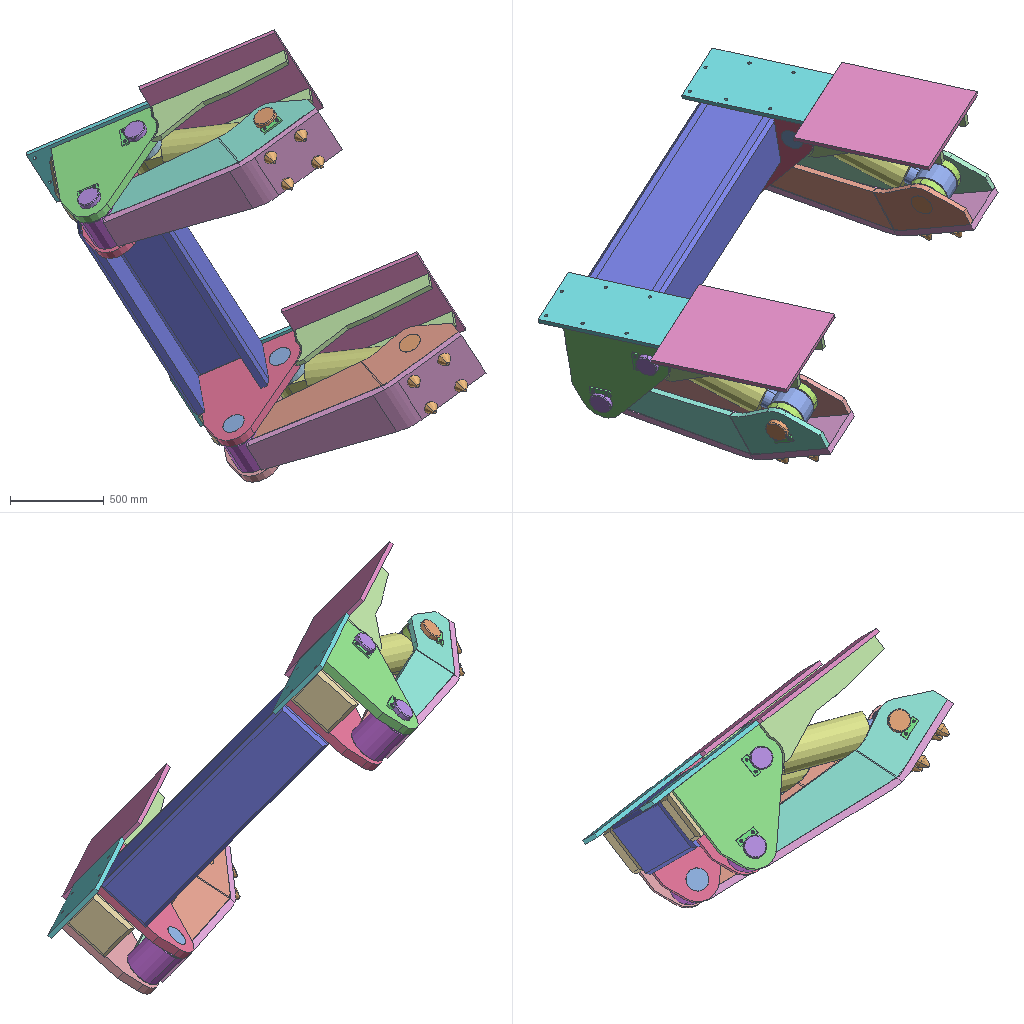Assembly | SolidWorks | 28 different items | 64 placed | box 2455 x 2223 x 2416 mm
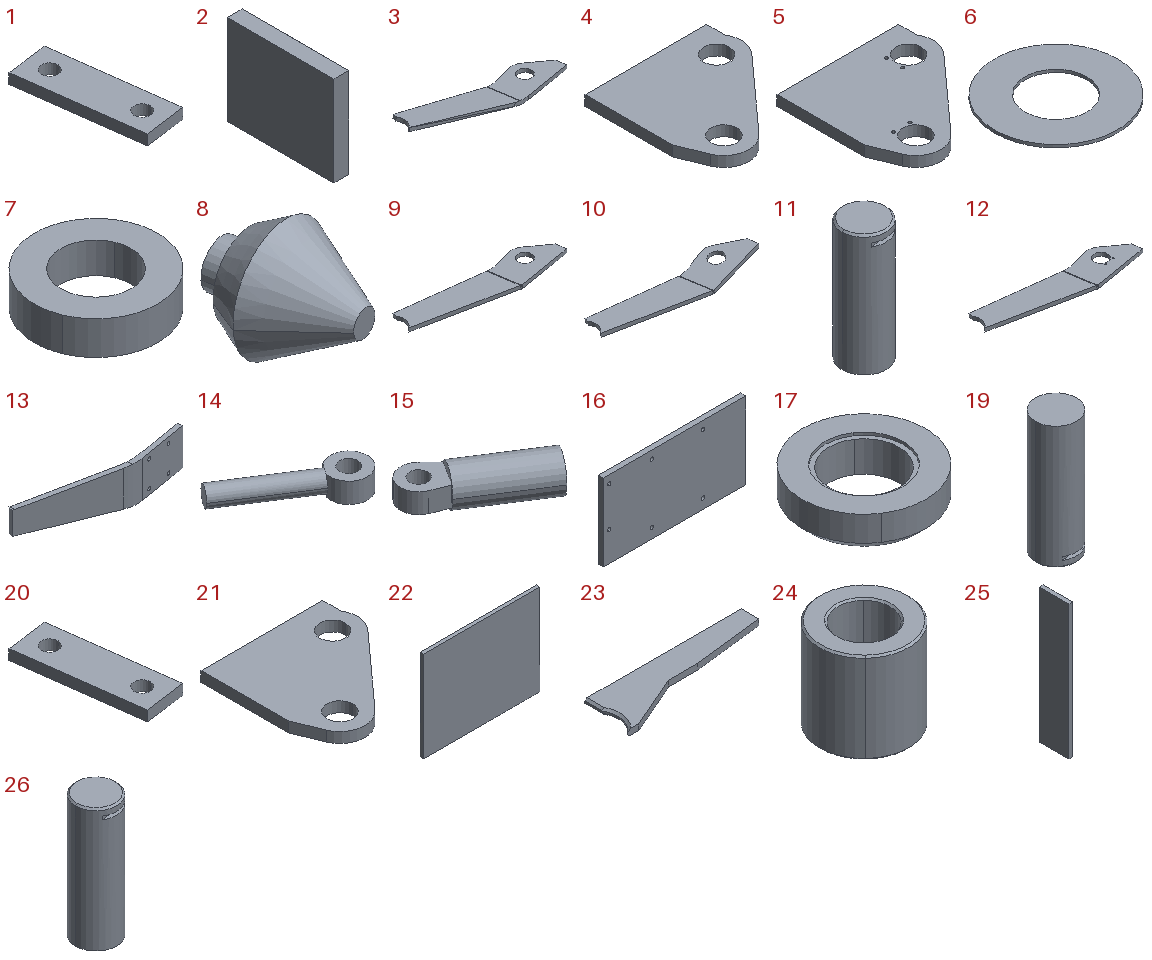Parts list (item | name | quantity | size | volume | features):
1 | - | x4 | 55.334 x 124.197 x 10 mm | 43979 mm3 | features Extrusion 1
2 | - | x2 | 60 x 290 x 245 mm | 4059667 mm3 | features SplitBody 1
3 | - | x1 | 1274 x 411.811 x 95.912 mm | 8557362 mm3 | features SplitBody 1
4 | - | x2 | 605 x 625 x 50 mm | 12914226 mm3 | features SplitBody 1
5 | - | x1 | 605 x 625 x 50 mm | 12901911 mm3 | features Cut 1, SplitBody 1
6 | - | x4 | 220 x 220 x 5 mm | 142550 mm3 | features Extrusion 1
7 | - | x4 | 220 x 220 x 60 mm | 1528876 mm3 | features SplitBody 1
8 | - | x8 | 74.124 x 87.696 x 75.094 mm | 169557 mm3 | features SplitBody 1
9 | - | x1 | 1274 x 418.793 x 95.912 mm | 8572989 mm3 | features SplitBody 1
10 | - | x1 | 1270 x 419.262 x 182.493 mm | 8566832 mm3 | features Cut 1, DeleteBody 1, MirrorSolid 1, SplitBody 1
11 | - | x2 | 125 x 125 x 344 mm | 4209039 mm3 | features ICE 2, Chamfer 1, Extrusion 1, MoveFace 1
12 | - | x1 | 1274 x 418.793 x 95.912 mm | 8566832 mm3 | features Cut 1, SplitBody 1
13 | - | x2 | 1303 x 271.725 x 314 mm | 14705850 mm3 | features SplitBody 1
14 | - | x2 | 664.027 x 492.763 x 120 mm | 8319390 mm3 | features SplitBody 1
15 | - | x2 | 696.192 x 540.383 x 219 mm | 10939320 mm3 | features SplitBody 1
16 | - | x2 | 720 x 25 x 390 mm | 6983921 mm3 | features SplitBody 1
17 | - | x4 | 220 x 220 x 60 mm | 1454656 mm3 | features SplitBody 1
18 | - | x1 | - | - | -
19 | - | x2 | 125 x 125 x 375.881 mm | 4600278 mm3 | features MirrorStock 1
20 | - | x2 | 55.334 x 124.197 x 10 mm | 43979 mm3 | features MirrorStock 1
21 | - | x1 | 605 x 625 x 50 mm | 12901911 mm3 | features MirrorStock 1
22 | - | x2 | 800 x 25 x 624 mm | 12480000 mm3 | features SplitBody 1
23 | - | x4 | 823 x 246 x 30 mm | 3379824 mm3 | features SplitBody 1
24 | - | x2 | 220 x 220 x 222 mm | 5474696 mm3 | features SplitBody 1
25 | - | x3 | 60 x 330 x 1510 mm | 29172667 mm3 | features SplitBody 1
26 | - | x2 | 125 x 125 x 375.881 mm | 4600278 mm3 | features ICE 2, Chamfer 1, Extrusion 1
27 | hexagon head bolts-full thread gb | x1 | - | - | -
28 | plain washers--product grade c gb | x1 | - | - | -
Mates (type | each side: item.copy, entity, surface, feature):
Coincident | 3.1 face plane Base part-9CBE5A036B009023550661BF37A96C0E-1 | 13.1 face plane Base part-9CBE5A036B009023550661BF37A96C0E-1 | 3 times
Coincident | 13.1 face plane Base part-9CBE5A036B009023550661BF37A96C0E-1 | 12.1 face plane Base part-9CBE5A036B009023550661BF37A96C0E-1 | 3 times
Concentric | 17.1 edge | 12.1 face cylinder Base part-9CBE5A036B009023550661BF37A96C0E-1
Concentric | 13.1 face cylinder Base part-9CBE5A036B009023550661BF37A96C0E-1 | 8.1 face cone Base part-9CBE5A036B009023550661BF37A96C0E-1
Coincident | 13.1 face plane Base part-9CBE5A036B009023550661BF37A96C0E-1 | 8.1 face plane Base part-9CBE5A036B009023550661BF37A96C0E-1
Concentric | 13.1 face cylinder Base part-9CBE5A036B009023550661BF37A96C0E-1 | 8.2 edge
Coincident | 13.1 face plane Base part-9CBE5A036B009023550661BF37A96C0E-1 | 8.2 edge
Coincident | 13.1 edge | 8.3 face cylinder Base part-9CBE5A036B009023550661BF37A96C0E-1
Coincident | 13.1 face plane Base part-9CBE5A036B009023550661BF37A96C0E-1 | 8.4 edge
Coincident | 17.1 face plane Base part-9CBE5A036B009023550661BF37A96C0E-1 | 12.1 face plane Base part-9CBE5A036B009023550661BF37A96C0E-1
Coincident | 3.1 face plane Base part-9CBE5A036B009023550661BF37A96C0E-1 | 17.2 face plane Base part-9CBE5A036B009023550661BF37A96C0E-1
Coincident | 13.1 face plane Base part-9CBE5A036B009023550661BF37A96C0E-1 | 8.3 edge
Concentric | 13.1 edge | 8.4 face cylinder Base part-9CBE5A036B009023550661BF37A96C0E-1
Concentric | 3.1 face cylinder Base part-9CBE5A036B009023550661BF37A96C0E-1 | 6.1 edge
Concentric | 3.1 face cylinder Base part-9CBE5A036B009023550661BF37A96C0E-1 | 6.2 face cylinder Boss-Extrude3
Coincident | 17.1 face plane Base part-9CBE5A036B009023550661BF37A96C0E-1 | 6.2 face plane Boss-Extrude3
Concentric | 5.1 face cylinder Base part-9CBE5A036B009023550661BF37A96C0E-1 | 4.1 face cylinder Base part-9CBE5A036B009023550661BF37A96C0E-1
Coincident | 5.1 edge | 4.1 face plane Base part-9CBE5A036B009023550661BF37A96C0E-1
Coincident | 5.1 edge | 7.1 face cylinder Base part-9CBE5A036B009023550661BF37A96C0E-1
Coincident | 5.1 face plane Base part-9CBE5A036B009023550661BF37A96C0E-1 | 7.1 face plane Base part-9CBE5A036B009023550661BF37A96C0E-1
Concentric | 3.1 face cylinder Base part-9CBE5A036B009023550661BF37A96C0E-1 | 17.2 face cylinder Base part-9CBE5A036B009023550661BF37A96C0E-1
Concentric | 3.1 face cylinder Base part-9CBE5A036B009023550661BF37A96C0E-1 | 6.1 face cylinder Boss-Extrude3
Concentric | 14.1 face cylinder Base part-9CBE5A036B009023550661BF37A96C0E-1 | 12.1 face cylinder Base part-9CBE5A036B009023550661BF37A96C0E-1
Coincident | 14.1 face plane Base part-9CBE5A036B009023550661BF37A96C0E-1 | 6.2 face plane Boss-Extrude3
Coincident | 17.2 face plane Base part-9CBE5A036B009023550661BF37A96C0E-1 | 6.1 face plane Boss-Extrude3
Concentric | 3.1 face cylinder Base part-9CBE5A036B009023550661BF37A96C0E-1 | 14.1 face cylinder Base part-9CBE5A036B009023550661BF37A96C0E-1
Concentric | 14.1 face cylinder Base part-9CBE5A036B009023550661BF37A96C0E-1 | 15.1 face cylinder Base part-9CBE5A036B009023550661BF37A96C0E-1
Concentric | 4.1 face cylinder Base part-9CBE5A036B009023550661BF37A96C0E-1 | 7.2 face cylinder Base part-9CBE5A036B009023550661BF37A96C0E-1
Coincident | 4.1 face plane Base part-9CBE5A036B009023550661BF37A96C0E-1 | 7.2 face plane Base part-9CBE5A036B009023550661BF37A96C0E-1
Parallel | 13.1 face plane Base part-9CBE5A036B009023550661BF37A96C0E-1 | 5.1 face plane Base part-9CBE5A036B009023550661BF37A96C0E-1
Lock | 13.1 select_type:0 | 24.1 select_type:0
Lock | 24.2 select_type:0 | 13.2 select_type:0
Concentric | 13.2 face cylinder Base part-9CBE5A036B009023550661BF37A96C0E-1 | 8.5 face cone Base part-9CBE5A036B009023550661BF37A96C0E-1
Concentric | 8.6 face cylinder Base part-9CBE5A036B009023550661BF37A96C0E-1 | 13.2 edge
Concentric | 9.1 face cylinder Base part-9CBE5A036B009023550661BF37A96C0E-1 | 17.3 edge
Concentric | 14.2 face cylinder Base part-9CBE5A036B009023550661BF37A96C0E-1 | 9.1 face cylinder Base part-9CBE5A036B009023550661BF37A96C0E-1
Concentric | 15.2 face cylinder Base part-9CBE5A036B009023550661BF37A96C0E-1 | 14.2 face cylinder Base part-9CBE5A036B009023550661BF37A96C0E-1
Concentric | 8.7 edge | 13.2 face cylinder Base part-9CBE5A036B009023550661BF37A96C0E-1
Coincident | 6.3 face plane Boss-Extrude3 | 17.3 face plane Base part-9CBE5A036B009023550661BF37A96C0E-1
Coincident | 13.2 face plane Base part-9CBE5A036B009023550661BF37A96C0E-1 | 9.1 face plane Base part-9CBE5A036B009023550661BF37A96C0E-1 | 3 times
Coincident | 8.7 edge | 13.2 face plane Base part-9CBE5A036B009023550661BF37A96C0E-1
Coincident | 13.2 face plane Base part-9CBE5A036B009023550661BF37A96C0E-1 | 8.5 face plane Base part-9CBE5A036B009023550661BF37A96C0E-1
Coincident | 13.2 edge | 8.8 face cylinder Base part-9CBE5A036B009023550661BF37A96C0E-1
Coincident | 8.6 edge | 13.2 face plane Base part-9CBE5A036B009023550661BF37A96C0E-1
Coincident | 9.1 face plane Base part-9CBE5A036B009023550661BF37A96C0E-1 | 17.3 face plane Base part-9CBE5A036B009023550661BF37A96C0E-1
Coincident | 7.3 face cylinder Base part-9CBE5A036B009023550661BF37A96C0E-1 | 4.2 edge
Coincident | 13.2 face plane Base part-9CBE5A036B009023550661BF37A96C0E-1 | 8.8 edge
Coincident | 6.3 face plane Boss-Extrude3 | 14.2 face plane Base part-9CBE5A036B009023550661BF37A96C0E-1
Coincident | 7.3 face plane Base part-9CBE5A036B009023550661BF37A96C0E-1 | 4.2 face plane Base part-9CBE5A036B009023550661BF37A96C0E-1
Coincident | 6.4 face plane Boss-Extrude3 | 17.4 face plane Base part-9CBE5A036B009023550661BF37A96C0E-1
Parallel | 13.2 face plane Base part-9CBE5A036B009023550661BF37A96C0E-1 | 4.2 face plane Base part-9CBE5A036B009023550661BF37A96C0E-1
Concentric | 15.1 edge | 15.2 edge
Concentric | 24.1 axis | 24.2 face cylinder Base part-9CBE5A036B009023550661BF37A96C0E-1
Parallel | 5.1 face plane Base part-9CBE5A036B009023550661BF37A96C0E-1 | 4.2 edge
Concentric | 12.1 edge | 9.1 edge
Coincident | 4.1 face plane Base part-9CBE5A036B009023550661BF37A96C0E-1 | 25.1 face plane Base part-9CBE5A036B009023550661BF37A96C0E-1 | 2 times
Coincident | 25.1 face plane Base part-9CBE5A036B009023550661BF37A96C0E-1 | 25.2 face plane Base part-9CBE5A036B009023550661BF37A96C0E-1 | 3 times
Coincident | 4.1 face plane Base part-9CBE5A036B009023550661BF37A96C0E-1 | 25.2 face plane Base part-9CBE5A036B009023550661BF37A96C0E-1
Coincident | 4.2 face plane Base part-9CBE5A036B009023550661BF37A96C0E-1 | 25.1 face plane Base part-9CBE5A036B009023550661BF37A96C0E-1
Coincident | 5.1 face plane Base part-9CBE5A036B009023550661BF37A96C0E-1 | 23.1 face plane Base part-9CBE5A036B009023550661BF37A96C0E-1 | 2 times
Concentric | 5.1 face cylinder Base part-9CBE5A036B009023550661BF37A96C0E-1 | 23.1 face cylinder Base part-9CBE5A036B009023550661BF37A96C0E-1
Coincident | 23.2 face plane Base part-9CBE5A036B009023550661BF37A96C0E-1 | 4.1 face plane Base part-9CBE5A036B009023550661BF37A96C0E-1
Coincident | 4.1 face plane Base part-9CBE5A036B009023550661BF37A96C0E-1 | 23.2 face plane Base part-9CBE5A036B009023550661BF37A96C0E-1 | 2 times
Parallel | 5.1 face plane Base part-9CBE5A036B009023550661BF37A96C0E-1 | 22.1 face plane Base part-9CBE5A036B009023550661BF37A96C0E-1
Coincident | 5.1 face plane Base part-9CBE5A036B009023550661BF37A96C0E-1 | 22.1 face plane Base part-9CBE5A036B009023550661BF37A96C0E-1
Coincident | 4.2 face plane Base part-9CBE5A036B009023550661BF37A96C0E-1 | 23.3 face plane Base part-9CBE5A036B009023550661BF37A96C0E-1 | 3 times
Coincident | 22.1 face plane Base part-9CBE5A036B009023550661BF37A96C0E-1 | 22.2 face plane Base part-9CBE5A036B009023550661BF37A96C0E-1
Coincident | 22.1 face plane Base part-9CBE5A036B009023550661BF37A96C0E-1 | 16.1 face plane Base part-9CBE5A036B009023550661BF37A96C0E-1
Coincident | 25.1 edge | 16.1 face plane Base part-9CBE5A036B009023550661BF37A96C0E-1
Coincident | 22.2 face plane Base part-9CBE5A036B009023550661BF37A96C0E-1 | 16.2 face plane Base part-9CBE5A036B009023550661BF37A96C0E-1
Coincident | 25.1 edge | 16.2 face plane Base part-9CBE5A036B009023550661BF37A96C0E-1
Coincident | 25.1 face plane Base part-9CBE5A036B009023550661BF37A96C0E-1 | 25.3 face plane Base part-9CBE5A036B009023550661BF37A96C0E-1 | 2 times
Coincident | 4.2 face plane Base part-9CBE5A036B009023550661BF37A96C0E-1 | 25.3 face plane Base part-9CBE5A036B009023550661BF37A96C0E-1
Coincident | 25.3 face plane Base part-9CBE5A036B009023550661BF37A96C0E-1 | 2.1 face plane Base part-9CBE5A036B009023550661BF37A96C0E-1
Coincident | 4.2 face plane Base part-9CBE5A036B009023550661BF37A96C0E-1 | 2.1 face plane Base part-9CBE5A036B009023550661BF37A96C0E-1
Coincident | 16.2 face plane Base part-9CBE5A036B009023550661BF37A96C0E-1 | 2.1 face plane Base part-9CBE5A036B009023550661BF37A96C0E-1
Coincident | 25.3 face plane Base part-9CBE5A036B009023550661BF37A96C0E-1 | 2.2 face plane Base part-9CBE5A036B009023550661BF37A96C0E-1
Coincident | 5.1 face plane Base part-9CBE5A036B009023550661BF37A96C0E-1 | 2.2 face plane Base part-9CBE5A036B009023550661BF37A96C0E-1
Coincident | 16.1 face plane Base part-9CBE5A036B009023550661BF37A96C0E-1 | 2.2 face plane Base part-9CBE5A036B009023550661BF37A96C0E-1
Width | 5.1 face plane Base part-9CBE5A036B009023550661BF37A96C0E-1 | 4.1 face plane Base part-9CBE5A036B009023550661BF37A96C0E-1 | 24.1 face plane Base part-9CBE5A036B009023550661BF37A96C0E-1 | 24.1 face plane Base part-9CBE5A036B009023550661BF37A96C0E-1
Concentric | 5.1 face cylinder Base part-9CBE5A036B009023550661BF37A96C0E-1 | 24.1 face cylinder Base part-9CBE5A036B009023550661BF37A96C0E-1
Concentric | 5.1 face cylinder Base part-9CBE5A036B009023550661BF37A96C0E-1 | 15.1 face cylinder Base part-9CBE5A036B009023550661BF37A96C0E-1
DistanceDim | 4.1 face plane Base part-9CBE5A036B009023550661BF37A96C0E-1 | 5.1 face plane Base part-9CBE5A036B009023550661BF37A96C0E-1
Concentric | 5.1 face cylinder Base part-9CBE5A036B009023550661BF37A96C0E-1 | 26.1 face cylinder Boss-Extrude1
Coincident | 5.1 face plane Base part-9CBE5A036B009023550661BF37A96C0E-1 | 26.1 face plane Boss-Extrude1
Parallel | 5.1 face plane Base part-9CBE5A036B009023550661BF37A96C0E-1 | 26.1 face plane Boss-Extrude2
Concentric | 5.1 face cylinder Base part-9CBE5A036B009023550661BF37A96C0E-1 | 26.2 face cylinder Boss-Extrude1
Coincident | 5.1 face plane Base part-9CBE5A036B009023550661BF37A96C0E-1 | 26.2 face plane Boss-Extrude1
Parallel | 16.1 face plane Base part-9CBE5A036B009023550661BF37A96C0E-1 | 26.2 face plane Boss-Extrude2
Coincident | 5.1 face plane Base part-9CBE5A036B009023550661BF37A96C0E-1 | 1.1 face plane Boss-Extrude1
Coincident | 26.2 face plane Boss-Extrude2 | 1.1 face plane Boss-Extrude1
Concentric | 5.1 face cylinder Cut-Extrude1 | 1.1 face cylinder Boss-Extrude1
Concentric | 5.1 face cylinder Cut-Extrude1 | 1.2 face cylinder Boss-Extrude1 | 2 times
Coincident | 5.1 face plane Base part-9CBE5A036B009023550661BF37A96C0E-1 | 1.2 face plane Boss-Extrude1
LimitPlanarAngleDim | 13.1 face plane Base part-9CBE5A036B009023550661BF37A96C0E-1 | 5.1 face plane Base part-9CBE5A036B009023550661BF37A96C0E-1
Concentric | 12.1 face cylinder Base part-9CBE5A036B009023550661BF37A96C0E-1 | 11.1 face cylinder Boss-Extrude1
Coincident | 3.1 face plane Base part-9CBE5A036B009023550661BF37A96C0E-1 | 11.1 face plane Boss-Extrude1
Parallel | 13.1 face plane Base part-9CBE5A036B009023550661BF37A96C0E-1 | 11.1 face plane Boss-Extrude2
Coincident | 12.1 face plane Base part-9CBE5A036B009023550661BF37A96C0E-1 | 1.3 face plane Boss-Extrude1
Concentric | 12.1 face cylinder Cut-Extrude1 | 1.3 face cylinder Boss-Extrude1 | 2 times
Coincident | 13.2 face plane Base part-9CBE5A036B009023550661BF37A96C0E-1 | 10.1 face plane Mirror1 | 2 times
Concentric | 10.1 face cylinder Mirror1 | 9.1 face cylinder Base part-9CBE5A036B009023550661BF37A96C0E-1
Concentric | 10.1 face cylinder Mirror1 | 17.4 face cylinder Base part-9CBE5A036B009023550661BF37A96C0E-1
Width | 4.2 face plane Base part-9CBE5A036B009023550661BF37A96C0E-1 | 21.1 face plane Rear Bracket with Two Holes1_Mirror | 24.2 face plane Base part-9CBE5A036B009023550661BF37A96C0E-1 | 24.2 face plane Base part-9CBE5A036B009023550661BF37A96C0E-1
Concentric | 6.3 face cylinder Boss-Extrude3 | 17.3 face cylinder Base part-9CBE5A036B009023550661BF37A96C0E-1
Concentric | 6.4 face cylinder Boss-Extrude3 | 17.4 face cylinder Base part-9CBE5A036B009023550661BF37A96C0E-1
Coincident | 10.1 face plane Mirror1 | 17.4 face plane Base part-9CBE5A036B009023550661BF37A96C0E-1
Coincident | 10.1 face plane Mirror1 | 1.4 face plane Boss-Extrude1
Concentric | 10.1 face cylinder Mirror1 | 1.4 face cylinder Boss-Extrude1 | 2 times
Concentric | 10.1 face cylinder Mirror1 | 11.2 face cylinder Boss-Extrude1
Coincident | 1.4 face plane Boss-Extrude1 | 11.2 face plane Boss-Extrude3
Parallel | 1.4 face plane Boss-Extrude1 | 11.2 face plane Boss-Extrude2
Coincident | 4.2 face plane Base part-9CBE5A036B009023550661BF37A96C0E-1 | 16.2 face plane Base part-9CBE5A036B009023550661BF37A96C0E-1